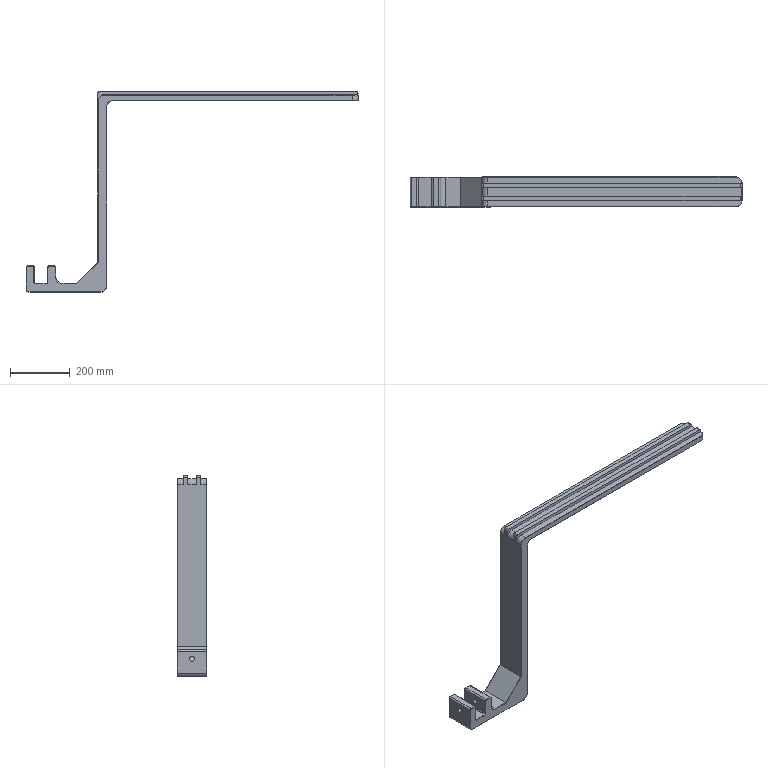Part | SolidWorks | features Fillet 6, ICE 3, Chamfer 2, Extrusion 1, MoveFace 1 | 1 solid | 106 faces | box 1110 x 100 x 669.85 mm | volume 5186013 mm3 | plane 57 | cone 26 | cylinder 23 | commonest cylinder face diameters 10 x8 40 x8 16 x4 4 x2 20 x1